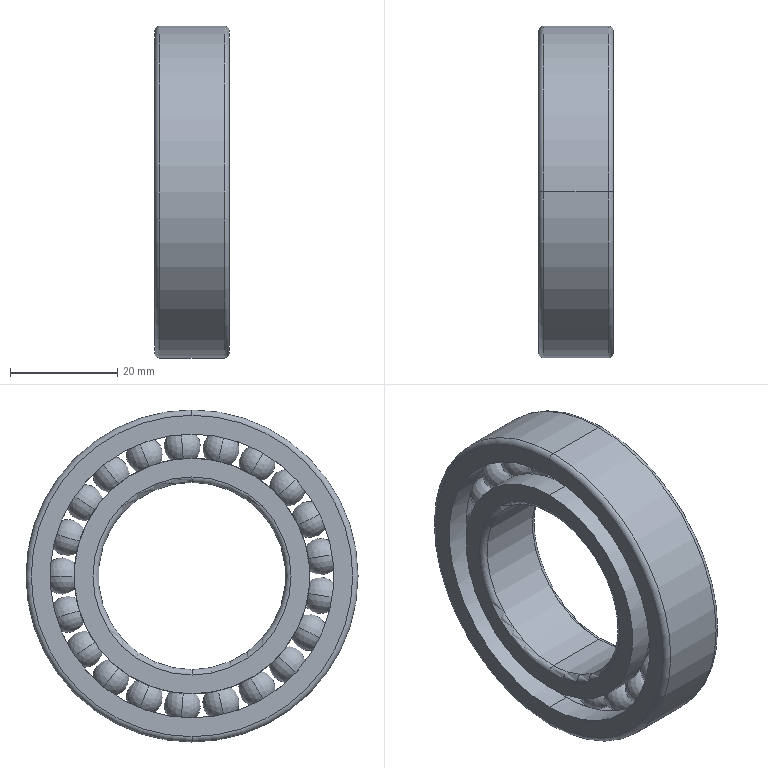Part | STEP file | deep groove ball bearings gb._Rolling bearings 6007 GB 276-94 | 1 solid | 132 faces | box 14 x 62 x 62 mm | volume 21271 mm3 | torus 74 | sphere 42 | cylinder 12 | plane 4 | commonest cylinder face diameters 44 x4 53 x4 35 x2 62 x2